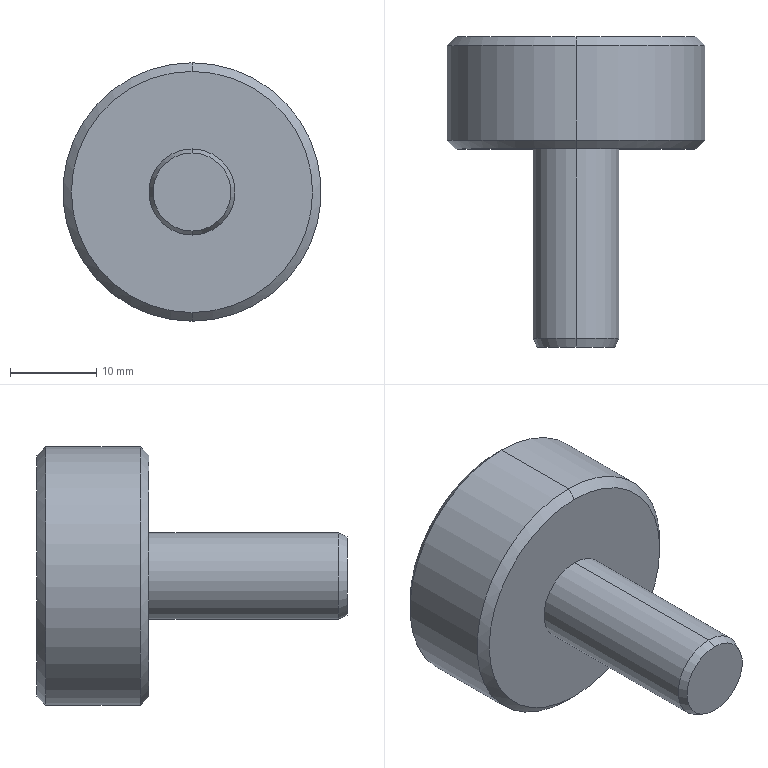Part | SolidWorks | features BaseBody 1 | 1 solid | 13 faces | box 30 x 36 x 30 mm | volume 10896 mm3 | cone 6 | cylinder 4 | plane 3 | commonest cylinder face diameters 10 x2 30 x2
STEP:
#1=CARTESIAN_POINT('',(418.,-42.,211.121));
#2=VERTEX_POINT('',#1);
#3=CARTESIAN_POINT('',(418.,-42.,183.121));
#4=VERTEX_POINT('',#3);
#5=CARTESIAN_POINT('',(418.,-42.,197.121));
#6=DIRECTION('',(0.,1.,0.));
#7=DIRECTION('',(0.,0.,-1.));
#8=AXIS2_PLACEMENT_3D('',#5,#6,#7);
#9=CIRCLE('',#8,14.);
#10=EDGE_CURVE('',#2,#4,#9,.T.);
#11=ORIENTED_EDGE('',*,*,#10,.F.);
#12=CARTESIAN_POINT('',(418.,-43.,212.121));
#13=VERTEX_POINT('',#12);
#14=CARTESIAN_POINT('',(418.,-43.,212.121));
#15=DIRECTION('',(0.,-0.7071,0.7071));
#16=VECTOR('',#15,1000.);
#17=LINE('',#14,#16);
#18=EDGE_CURVE('',#2,#13,#17,.T.);
#19=ORIENTED_EDGE('',*,*,#18,.T.);
#20=CARTESIAN_POINT('',(418.,-43.,182.121));
#21=VERTEX_POINT('',#20);
#22=CARTESIAN_POINT('',(418.,-43.,197.121));
#23=DIRECTION('',(0.,1.,0.));
#24=DIRECTION('',(-1.,0.,0.));
#25=AXIS2_PLACEMENT_3D('',#22,#23,#24);
#26=CIRCLE('',#25,15.);
#27=EDGE_CURVE('',#13,#21,#26,.T.);
#28=ORIENTED_EDGE('',*,*,#27,.T.);
#29=CARTESIAN_POINT('',(418.,-43.,182.121));
#30=DIRECTION('',(0.,-0.7071,-0.7071));
#31=VECTOR('',#30,1000.);
#32=LINE('',#29,#31);
#33=EDGE_CURVE('',#4,#21,#32,.T.);
#34=ORIENTED_EDGE('',*,*,#33,.F.);
#35=EDGE_LOOP('',(#11,#19,#28,#34));
#36=FACE_OUTER_BOUND('',#35,.T.);
#37=CARTESIAN_POINT('',(418.,-43.,197.121));
#38=DIRECTION('',(0.,-1.,0.));
#39=DIRECTION('',(0.,0.,-1.));
#40=AXIS2_PLACEMENT_3D('',#37,#38,#39);
#41=CONICAL_SURFACE('',#40,15.,0.7854);
#42=ADVANCED_FACE('',(#36),#41,.T.);
#43=ORIENTED_EDGE('',*,*,#27,.F.);
#44=CARTESIAN_POINT('',(418.,-54.,212.121));
#45=VERTEX_POINT('',#44);
#46=CARTESIAN_POINT('',(418.,-78.,212.121));
#47=DIRECTION('',(0.,-1.,0.));
#48=VECTOR('',#47,1000.);
#49=LINE('',#46,#48);
#50=EDGE_CURVE('',#13,#45,#49,.T.);
#51=ORIENTED_EDGE('',*,*,#50,.T.);
#52=CARTESIAN_POINT('',(418.,-54.,182.121));
#53=VERTEX_POINT('',#52);
#54=CARTESIAN_POINT('',(418.,-54.,197.121));
#55=DIRECTION('',(0.,1.,0.));
#56=DIRECTION('',(0.,0.,-1.));
#57=AXIS2_PLACEMENT_3D('',#54,#55,#56);
#58=CIRCLE('',#57,15.);
#59=EDGE_CURVE('',#45,#53,#58,.T.);
#60=ORIENTED_EDGE('',*,*,#59,.T.);
#61=CARTESIAN_POINT('',(418.,-78.,182.121));
#62=DIRECTION('',(0.,-1.,0.));
#63=VECTOR('',#62,1000.);
#64=LINE('',#61,#63);
#65=EDGE_CURVE('',#21,#53,#64,.T.);
#66=ORIENTED_EDGE('',*,*,#65,.F.);
#67=EDGE_LOOP('',(#43,#51,#60,#66));
#68=FACE_OUTER_BOUND('',#67,.T.);
#69=CARTESIAN_POINT('',(418.,-78.,197.121));
#70=DIRECTION('',(0.,-1.,0.));
#71=DIRECTION('',(0.,0.,-1.));
#72=AXIS2_PLACEMENT_3D('',#69,#70,#71);
#73=CYLINDRICAL_SURFACE('',#72,15.);
#74=ADVANCED_FACE('',(#68),#73,.T.);
#75=CARTESIAN_POINT('',(418.,-55.,211.121));
#76=VERTEX_POINT('',#75);
#77=CARTESIAN_POINT('',(418.,-55.,183.121));
#78=VERTEX_POINT('',#77);
#79=CARTESIAN_POINT('',(418.,-55.,197.121));
#80=DIRECTION('',(0.,1.,0.));
#81=DIRECTION('',(0.,0.,1.));
#82=AXIS2_PLACEMENT_3D('',#79,#80,#81);
#83=CIRCLE('',#82,14.);
#84=EDGE_CURVE('',#76,#78,#83,.T.);
#85=ORIENTED_EDGE('',*,*,#84,.T.);
#86=CARTESIAN_POINT('',(418.,-54.,182.121));
#87=DIRECTION('',(0.,0.7071,-0.7071));
#88=VECTOR('',#87,1000.);
#89=LINE('',#86,#88);
#90=EDGE_CURVE('',#78,#53,#89,.T.);
#91=ORIENTED_EDGE('',*,*,#90,.T.);
#92=ORIENTED_EDGE('',*,*,#59,.F.);
#93=CARTESIAN_POINT('',(418.,-54.,212.121));
#94=DIRECTION('',(0.,0.7071,0.7071));
#95=VECTOR('',#94,1000.);
#96=LINE('',#93,#95);
#97=EDGE_CURVE('',#76,#45,#96,.T.);
#98=ORIENTED_EDGE('',*,*,#97,.F.);
#99=EDGE_LOOP('',(#85,#91,#92,#98));
#100=FACE_OUTER_BOUND('',#99,.T.);
#101=CARTESIAN_POINT('',(418.,-54.,197.121));
#102=DIRECTION('',(0.,1.,0.));
#103=DIRECTION('',(0.,0.,1.));
#104=AXIS2_PLACEMENT_3D('',#101,#102,#103);
#105=CONICAL_SURFACE('',#104,15.,0.7854);
#106=ADVANCED_FACE('',(#100),#105,.T.);
#107=CARTESIAN_POINT('',(418.,-55.,202.121));
#108=VERTEX_POINT('',#107);
#109=CARTESIAN_POINT('',(418.,-55.,192.121));
#110=VERTEX_POINT('',#109);
#111=CARTESIAN_POINT('',(418.,-55.,197.121));
#112=DIRECTION('',(0.,1.,0.));
#113=DIRECTION('',(0.,0.,-1.));
#114=AXIS2_PLACEMENT_3D('',#111,#112,#113);
#115=CIRCLE('',#114,5.);
#116=EDGE_CURVE('',#108,#110,#115,.T.);
#117=ORIENTED_EDGE('',*,*,#116,.F.);
#118=CARTESIAN_POINT('',(418.,-77.,202.121));
#119=VERTEX_POINT('',#118);
#120=CARTESIAN_POINT('',(418.,-78.,202.121));
#121=DIRECTION('',(0.,-1.,0.));
#122=VECTOR('',#121,1000.);
#123=LINE('',#120,#122);
#124=EDGE_CURVE('',#108,#119,#123,.T.);
#125=ORIENTED_EDGE('',*,*,#124,.T.);
#126=CARTESIAN_POINT('',(418.,-77.,192.121));
#127=VERTEX_POINT('',#126);
#128=CARTESIAN_POINT('',(418.,-77.,197.121));
#129=DIRECTION('',(0.,1.,0.));
#130=DIRECTION('',(0.,0.,-1.));
#131=AXIS2_PLACEMENT_3D('',#128,#129,#130);
#132=CIRCLE('',#131,5.);
#133=EDGE_CURVE('',#119,#127,#132,.T.);
#134=ORIENTED_EDGE('',*,*,#133,.T.);
#135=CARTESIAN_POINT('',(418.,-78.,192.121));
#136=DIRECTION('',(0.,-1.,0.));
#137=VECTOR('',#136,1000.);
#138=LINE('',#135,#137);
#139=EDGE_CURVE('',#110,#127,#138,.T.);
#140=ORIENTED_EDGE('',*,*,#139,.F.);
#141=EDGE_LOOP('',(#117,#125,#134,#140));
#142=FACE_OUTER_BOUND('',#141,.T.);
#143=CARTESIAN_POINT('',(418.,-78.,197.121));
#144=DIRECTION('',(0.,-1.,0.));
#145=DIRECTION('',(0.,0.,-1.));
#146=AXIS2_PLACEMENT_3D('',#143,#144,#145);
#147=CYLINDRICAL_SURFACE('',#146,5.);
#148=ADVANCED_FACE('',(#142),#147,.T.);
#149=CARTESIAN_POINT('',(418.,-78.,201.655));
#150=VERTEX_POINT('',#149);
#151=CARTESIAN_POINT('',(418.,-78.,192.587));
#152=VERTEX_POINT('',#151);
#153=CARTESIAN_POINT('',(418.,-78.,197.121));
#154=DIRECTION('',(0.,1.,0.));
#155=DIRECTION('',(0.,0.,1.));
#156=AXIS2_PLACEMENT_3D('',#153,#154,#155);
#157=CIRCLE('',#156,4.534);
#158=EDGE_CURVE('',#150,#152,#157,.T.);
#159=ORIENTED_EDGE('',*,*,#158,.T.);
#160=CARTESIAN_POINT('',(418.,-77.,192.121));
#161=DIRECTION('',(0.,0.9063,-0.4226));
#162=VECTOR('',#161,1000.);
#163=LINE('',#160,#162);
#164=EDGE_CURVE('',#152,#127,#163,.T.);
#165=ORIENTED_EDGE('',*,*,#164,.T.);
#166=ORIENTED_EDGE('',*,*,#133,.F.);
#167=CARTESIAN_POINT('',(418.,-77.,202.121));
#168=DIRECTION('',(0.,0.9063,0.4226));
#169=VECTOR('',#168,1000.);
#170=LINE('',#167,#169);
#171=EDGE_CURVE('',#150,#119,#170,.T.);
#172=ORIENTED_EDGE('',*,*,#171,.F.);
#173=EDGE_LOOP('',(#159,#165,#166,#172));
#174=FACE_OUTER_BOUND('',#173,.T.);
#175=CARTESIAN_POINT('',(418.,-77.,197.121));
#176=DIRECTION('',(0.,1.,0.));
#177=DIRECTION('',(0.,0.,1.));
#178=AXIS2_PLACEMENT_3D('',#175,#176,#177);
#179=CONICAL_SURFACE('',#178,5.,0.4363);
#180=ADVANCED_FACE('',(#174),#179,.T.);
#181=CARTESIAN_POINT('',(418.,-42.,197.121));
#182=DIRECTION('',(0.,1.,0.));
#183=DIRECTION('',(0.,0.,-1.));
#184=AXIS2_PLACEMENT_3D('',#181,#182,#183);
#185=CIRCLE('',#184,14.);
#186=EDGE_CURVE('',#4,#2,#185,.T.);
#187=ORIENTED_EDGE('',*,*,#186,.T.);
#188=ORIENTED_EDGE('',*,*,#10,.T.);
#189=EDGE_LOOP('',(#187,#188));
#190=FACE_OUTER_BOUND('',#189,.T.);
#191=CARTESIAN_POINT('',(418.,-42.,197.121));
#192=DIRECTION('',(0.,1.,0.));
#193=DIRECTION('',(0.,0.,1.));
#194=AXIS2_PLACEMENT_3D('',#191,#192,#193);
#195=PLANE('',#194);
#196=ADVANCED_FACE('',(#190),#195,.T.);
#197=ORIENTED_EDGE('',*,*,#18,.F.);
#198=ORIENTED_EDGE('',*,*,#186,.F.);
#199=ORIENTED_EDGE('',*,*,#33,.T.);
#200=CARTESIAN_POINT('',(418.,-43.,197.121));
#201=DIRECTION('',(0.,1.,0.));
#202=DIRECTION('',(-1.,0.,0.));
#203=AXIS2_PLACEMENT_3D('',#200,#201,#202);
#204=CIRCLE('',#203,15.);
#205=EDGE_CURVE('',#21,#13,#204,.T.);
#206=ORIENTED_EDGE('',*,*,#205,.T.);
#207=EDGE_LOOP('',(#197,#198,#199,#206));
#208=FACE_OUTER_BOUND('',#207,.T.);
#209=CARTESIAN_POINT('',(418.,-43.,197.121));
#210=DIRECTION('',(0.,-1.,0.));
#211=DIRECTION('',(0.,0.,-1.));
#212=AXIS2_PLACEMENT_3D('',#209,#210,#211);
#213=CONICAL_SURFACE('',#212,15.,0.7854);
#214=ADVANCED_FACE('',(#208),#213,.T.);
#215=ORIENTED_EDGE('',*,*,#50,.F.);
#216=ORIENTED_EDGE('',*,*,#205,.F.);
#217=ORIENTED_EDGE('',*,*,#65,.T.);
#218=CARTESIAN_POINT('',(418.,-54.,197.121));
#219=DIRECTION('',(0.,1.,0.));
#220=DIRECTION('',(0.,0.,-1.));
#221=AXIS2_PLACEMENT_3D('',#218,#219,#220);
#222=CIRCLE('',#221,15.);
#223=EDGE_CURVE('',#53,#45,#222,.T.);
#224=ORIENTED_EDGE('',*,*,#223,.T.);
#225=EDGE_LOOP('',(#215,#216,#217,#224));
#226=FACE_OUTER_BOUND('',#225,.T.);
#227=CARTESIAN_POINT('',(418.,-78.,197.121));
#228=DIRECTION('',(0.,-1.,0.));
#229=DIRECTION('',(0.,0.,-1.));
#230=AXIS2_PLACEMENT_3D('',#227,#228,#229);
#231=CYLINDRICAL_SURFACE('',#230,15.);
#232=ADVANCED_FACE('',(#226),#231,.T.);
#233=ORIENTED_EDGE('',*,*,#90,.F.);
#234=CARTESIAN_POINT('',(418.,-55.,197.121));
#235=DIRECTION('',(0.,1.,0.));
#236=DIRECTION('',(0.,0.,1.));
#237=AXIS2_PLACEMENT_3D('',#234,#235,#236);
#238=CIRCLE('',#237,14.);
#239=EDGE_CURVE('',#78,#76,#238,.T.);
#240=ORIENTED_EDGE('',*,*,#239,.T.);
#241=ORIENTED_EDGE('',*,*,#97,.T.);
#242=ORIENTED_EDGE('',*,*,#223,.F.);
#243=EDGE_LOOP('',(#233,#240,#241,#242));
#244=FACE_OUTER_BOUND('',#243,.T.);
#245=CARTESIAN_POINT('',(418.,-54.,197.121));
#246=DIRECTION('',(0.,1.,0.));
#247=DIRECTION('',(0.,0.,1.));
#248=AXIS2_PLACEMENT_3D('',#245,#246,#247);
#249=CONICAL_SURFACE('',#248,15.,0.7854);
#250=ADVANCED_FACE('',(#244),#249,.T.);
#251=CARTESIAN_POINT('',(418.,-55.,197.121));
#252=DIRECTION('',(0.,1.,0.));
#253=DIRECTION('',(0.,0.,-1.));
#254=AXIS2_PLACEMENT_3D('',#251,#252,#253);
#255=CIRCLE('',#254,5.);
#256=EDGE_CURVE('',#110,#108,#255,.T.);
#257=ORIENTED_EDGE('',*,*,#256,.T.);
#258=ORIENTED_EDGE('',*,*,#116,.T.);
#259=EDGE_LOOP('',(#257,#258));
#260=FACE_BOUND('',#259,.T.);
#261=ORIENTED_EDGE('',*,*,#84,.F.);
#262=ORIENTED_EDGE('',*,*,#239,.F.);
#263=EDGE_LOOP('',(#261,#262));
#264=FACE_OUTER_BOUND('',#263,.T.);
#265=CARTESIAN_POINT('',(403.,-55.,197.121));
#266=DIRECTION('',(0.,-1.,0.));
#267=DIRECTION('',(0.,0.,-1.));
#268=AXIS2_PLACEMENT_3D('',#265,#266,#267);
#269=PLANE('',#268);
#270=ADVANCED_FACE('',(#260,#264),#269,.T.);
#271=ORIENTED_EDGE('',*,*,#124,.F.);
#272=ORIENTED_EDGE('',*,*,#256,.F.);
#273=ORIENTED_EDGE('',*,*,#139,.T.);
#274=CARTESIAN_POINT('',(418.,-77.,197.121));
#275=DIRECTION('',(0.,1.,0.));
#276=DIRECTION('',(0.,0.,-1.));
#277=AXIS2_PLACEMENT_3D('',#274,#275,#276);
#278=CIRCLE('',#277,5.);
#279=EDGE_CURVE('',#127,#119,#278,.T.);
#280=ORIENTED_EDGE('',*,*,#279,.T.);
#281=EDGE_LOOP('',(#271,#272,#273,#280));
#282=FACE_OUTER_BOUND('',#281,.T.);
#283=CARTESIAN_POINT('',(418.,-78.,197.121));
#284=DIRECTION('',(0.,-1.,0.));
#285=DIRECTION('',(0.,0.,-1.));
#286=AXIS2_PLACEMENT_3D('',#283,#284,#285);
#287=CYLINDRICAL_SURFACE('',#286,5.);
#288=ADVANCED_FACE('',(#282),#287,.T.);
#289=ORIENTED_EDGE('',*,*,#164,.F.);
#290=CARTESIAN_POINT('',(418.,-78.,197.121));
#291=DIRECTION('',(0.,1.,0.));
#292=DIRECTION('',(0.,0.,1.));
#293=AXIS2_PLACEMENT_3D('',#290,#291,#292);
#294=CIRCLE('',#293,4.534);
#295=EDGE_CURVE('',#152,#150,#294,.T.);
#296=ORIENTED_EDGE('',*,*,#295,.T.);
#297=ORIENTED_EDGE('',*,*,#171,.T.);
#298=ORIENTED_EDGE('',*,*,#279,.F.);
#299=EDGE_LOOP('',(#289,#296,#297,#298));
#300=FACE_OUTER_BOUND('',#299,.T.);
#301=CARTESIAN_POINT('',(418.,-77.,197.121));
#302=DIRECTION('',(0.,1.,0.));
#303=DIRECTION('',(0.,0.,1.));
#304=AXIS2_PLACEMENT_3D('',#301,#302,#303);
#305=CONICAL_SURFACE('',#304,5.,0.4363);
#306=ADVANCED_FACE('',(#300),#305,.T.);
#307=ORIENTED_EDGE('',*,*,#158,.F.);
#308=ORIENTED_EDGE('',*,*,#295,.F.);
#309=EDGE_LOOP('',(#307,#308));
#310=FACE_OUTER_BOUND('',#309,.T.);
#311=CARTESIAN_POINT('',(413.,-78.,197.121));
#312=DIRECTION('',(0.,-1.,0.));
#313=DIRECTION('',(0.,0.,-1.));
#314=AXIS2_PLACEMENT_3D('',#311,#312,#313);
#315=PLANE('',#314);
#316=ADVANCED_FACE('',(#310),#315,.T.);
#317=CLOSED_SHELL('',(#42,#74,#106,#148,#180,#196,#214,#232,#250,#270,#288,#306,#316));
#318=MANIFOLD_SOLID_BREP('',#317);
#319=CARTESIAN_POINT('',(0.,0.,0.));
#320=DIRECTION('',(0.,0.,1.));
#321=DIRECTION('',(1.,0.,0.));
#322=AXIS2_PLACEMENT_3D('',#319,#320,#321);
#323=(LENGTH_UNIT()NAMED_UNIT(*)SI_UNIT(.MILLI.,.METRE.));
#324=UNCERTAINTY_MEASURE_WITH_UNIT(LENGTH_MEASURE(0.00001),#323,'','');
#325=(NAMED_UNIT(*)PLANE_ANGLE_UNIT()SI_UNIT($,.RADIAN.));
#326=(NAMED_UNIT(*)SI_UNIT($,.STERADIAN.)SOLID_ANGLE_UNIT());
#327=(GEOMETRIC_REPRESENTATION_CONTEXT(3)GLOBAL_UNCERTAINTY_ASSIGNED_CONTEXT((#324))GLOBAL_UNIT_ASSIGNED_CONTEXT((#323,#325,#326))REPRESENTATION_CONTEXT('',''));
#328=ADVANCED_BREP_SHAPE_REPRESENTATION('',(#318,#322),#327);